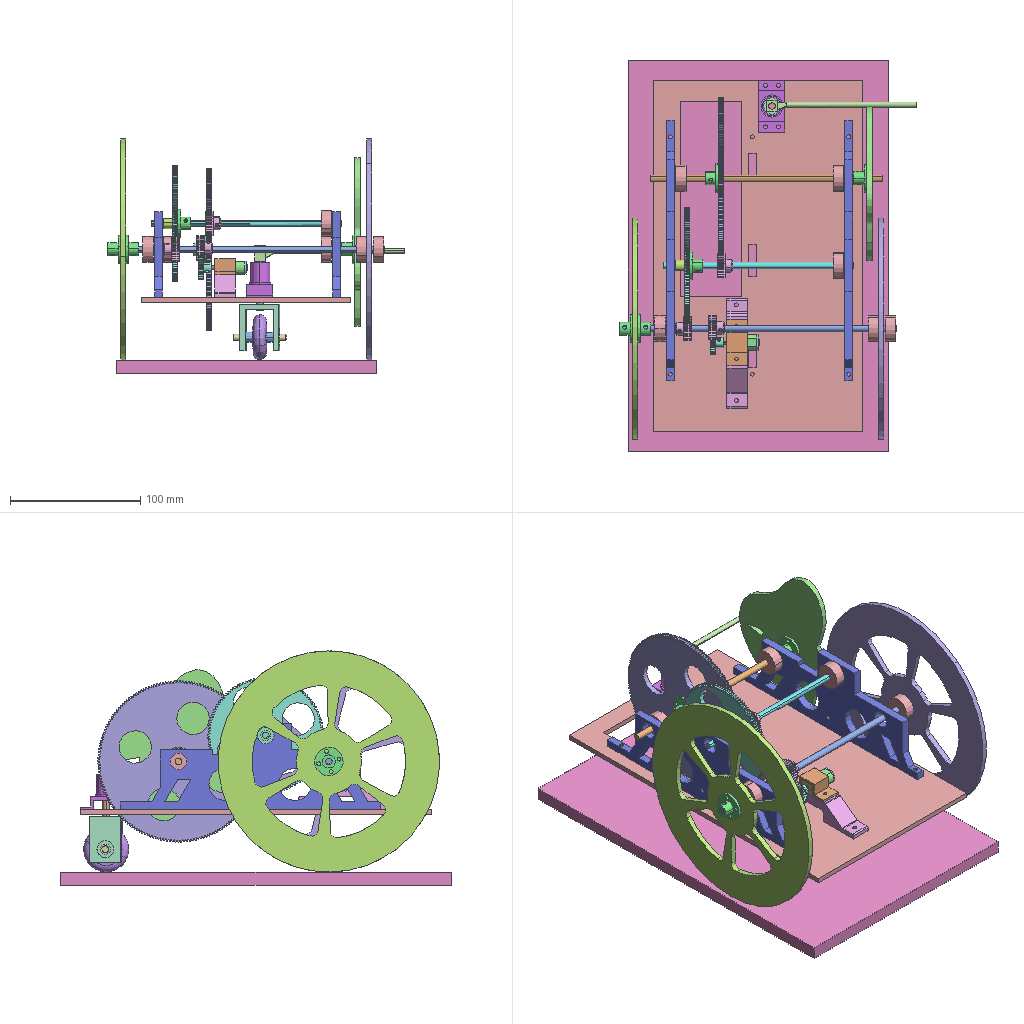Assembly | SolidWorks | 28 different items | 41 placed | box 228 x 300 x 180 mm
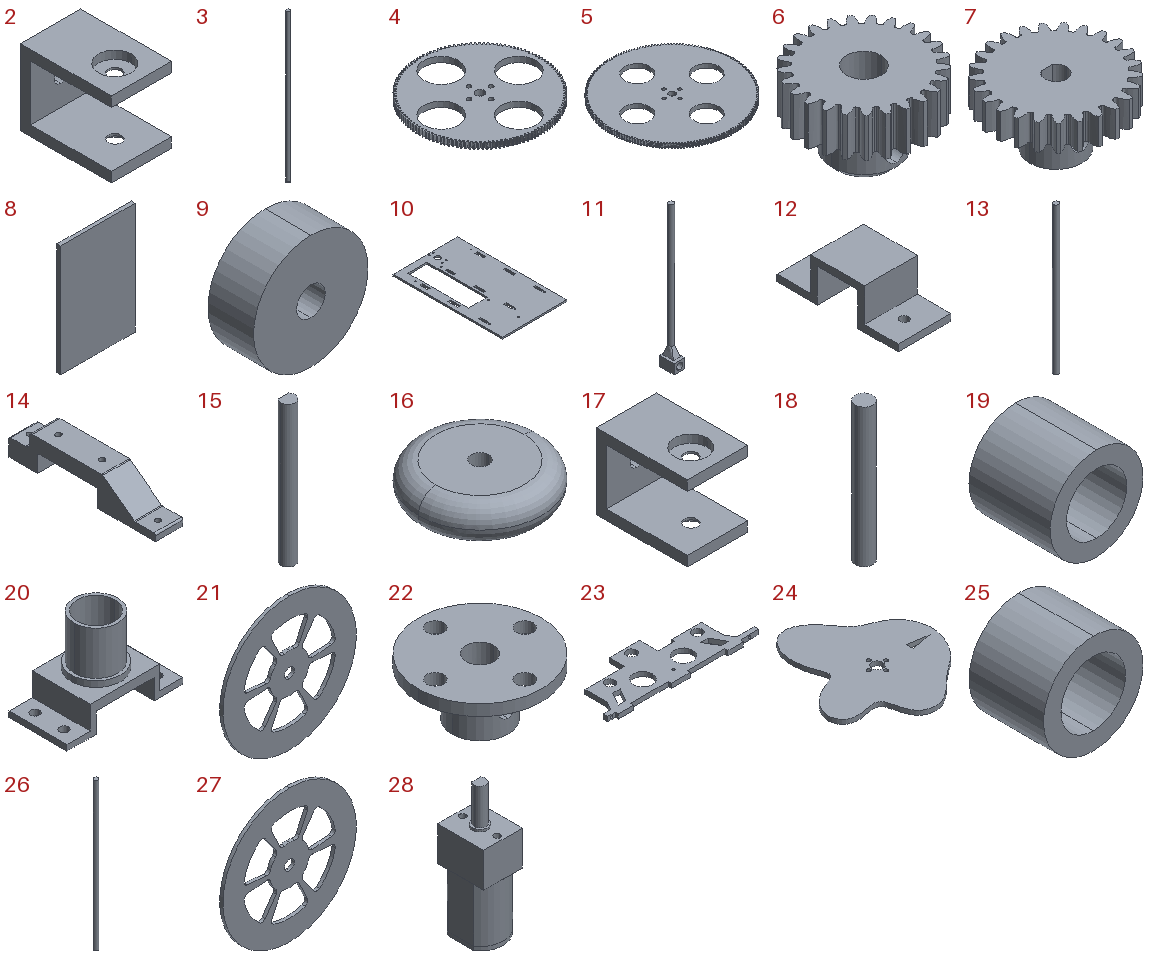Parts list (item | name | quantity | parent item | size | volume | features):
1 | (subassembly) | x1 | - | - | - | -
2 | (subassembly) | x1 | - | 23.897 x 36 x 30 mm | 8017 mm3 | -
3 | - | x1 | - | 5 x 5 x 213 mm | 3913 mm3 | features ICE 3, Extrusion 1
4 | - | x1 | - | 88.898 x 88.892 x 4 mm | 15932 mm3 | features ICE 8, CirPattern 1, Extrusion 1, RefAxis 1
5 | - | x1 | - | 123.899 x 123.895 x 4 mm | 39033 mm3 | features ICE 2, CirPattern 1, Extrusion 1, RefAxis 1
6 | - | x3 | - | 18.888 x 18.854 x 12 mm | 1581 mm3 | features ICE 6, Chamfer 1, CirPattern 1, Extrusion 1, RefAxis 1
7 | - | x1 | - | 18.888 x 18.854 x 10 mm | 1132 mm3 | features ICE 7, CirPattern 1, Extrusion 1, RefAxis 1
8 | - | x1 | - | 200 x 10 x 300 mm | 600000 mm3 | features Extrusion 1
9 | - | x6 | - | 20 x 8 x 20 mm | 2356 mm3 | features Extrusion 1
10 | - | x1 | - | 161 x 270 x 4 mm | 140085 mm3 | features ICE 34, FlatPattern 1, SMBaseFlange 1, SheetMetal 1
11 | - | x1 | - | 8.5 x 12 x 115 mm | 2022 mm3 | features ICE 4, Blend 1, Extrusion 1
12 | - | x1 | - | 15.7 x 36 x 12 mm | 1739 mm3 | features ICE 3, Extrusion 1, HoleWzd 1
13 | - | x1 | - | 5 x 5 x 146 mm | 2741 mm3 | features ICE 2, Extrusion 1
14 | - | x1 | - | 15.7 x 84.104 x 18.06 mm | 12021 mm3 | features ICE 11, Fillet 3, Extrusion 1
15 | - | x1 | - | 5 x 5 x 50 mm | 947.142 mm3 | features ICE 2, Extrusion 1
16 | - | x1 | - | 35 x 35 x 10 mm | 8320 mm3 | features Extrusion 1, Fillet 1, ICE 1
17 | - | x1 | in 2 | 23.897 x 36 x 30 mm | 8017 mm3 | features ICE 12, Extrusion 1, MirrorPattern 1
18 | - | x1 | - | 5 x 5 x 40 mm | 785.398 mm3 | features Extrusion 1
19 | - | x1 | - | 8 x 7 x 8 mm | 203.198 mm3 | features Extrusion 1
20 | - | x1 | - | 40 x 20 x 27 mm | 3033 mm3 | features ICE 9, Extrusion 1
21 | - | x1 | - | 170 x 4 x 170 mm | 60845 mm3 | features Extrusion 1, Fillet 1, ICE 1
22 | - | x5 | - | 22 x 22 x 10 mm | 1099 mm3 | features ICE 4, Extrusion 1
23 | - | x2 | - | 200 x 70 x 6 mm | 39858 mm3 | features ICE 11, Extrusion 1
24 | - | x1 | - | 117.822 x 129.451 x 4 mm | 34423 mm3 | features CurveInFile 1, Extrusion 1
25 | - | x2 | - | 8 x 6 x 8 mm | 174.17 mm3 | features Extrusion 1
26 | - | x1 | - | 5 x 5 x 178.5 mm | 3505 mm3 | features Extrusion 1
27 | - | x1 | - | 170 x 4 x 170 mm | 60862 mm3 | features Extrusion 1, Fillet 1, ICE 1
28 | - | x1 | - | 10 x 12 x 35 mm | 2719 mm3 | features MBimport 1
Mates (type | each side: item.copy, entity, surface, feature):
Coincident | 10.1 face plane Base-Flange1 | assembly face | 8 times
Coincident | 10.1 face plane Cut-Extrude1 | assembly face | 2 times
Coincident | 10.1 face | assembly face | 6 times
Coincident | assembly face | assembly face | 60 times
Concentric | assembly face | assembly face | 19 times
Concentric | assembly face | 3.1 face cylinder Boss-Extrude1 | 4 times
DistanceDim | 3.1 face plane Boss-Extrude1 | assembly face | 2 times
Concentric | 3.1 face cylinder Boss-Extrude1 | 27.1 face cylinder Boss-Extrude1
Concentric | 27.1 face cylinder Boss-Extrude1 | assembly face | 2 times
Coincident | 27.1 face plane Boss-Extrude1 | assembly face | 2 times
Concentric | 3.1 face cylinder Boss-Extrude1 | assembly face | 4 times
Concentric | 3.1 face cylinder Boss-Extrude1 | 6.1 face cylinder Cut-Extrude6
Coincident | assembly face | 6.1 face plane Boss-Extrude3
Coincident | 4.1 face plane Cut-Extrude2 | assembly face
Concentric | assembly face | 26.1 face cylinder Boss-Extrude1 | 4 times
DistanceDim | 26.1 face plane Boss-Extrude1 | assembly face
Coincident | assembly face | 6.2 face plane Boss-Extrude3
Coincident | 3.1 face plane Boss-Extrude1 | assembly face
Coincident | 10.1 face plane Cut-Extrude8 | assembly face | 2 times
Coincident | 6.2 face plane Boss-Extrude3 | assembly face
Concentric | 10.1 face | assembly face | 4 times
Concentric | 20.1 face cylinder Boss-Extrude1 | assembly face
Coincident | 20.1 face plane Boss-Extrude1 | assembly face
Concentric | assembly face | 15.1 face cylinder Boss-Extrude1
Coincident | 10.1 face plane Base-Flange1 | 23.1 face plane Cut-Extrude1
Coincident | assembly face | 23.1 face plane Boss-Extrude1 | 6 times
Coincident | 10.1 face plane Base-Flange1 | 23.2 face plane Cut-Extrude1
Coincident | assembly face | 23.2 face plane Boss-Extrude1 | 6 times
Coincident | 6.1 face plane Boss-Extrude3 | assembly face
Concentric | assembly face | 23.2 face cylinder Boss-Extrude2
Perpendicular | 3.1 face plane Cut-Extrude2 | 6.1 axis
Perpendicular | 3.1 face plane Cut-Extrude2 | 6.3 axis
GearDim | 4.1 face cylinder Boss-Extrude1 | 6.1 face cylinder CirPattern1
DistanceDim | 26.1 face plane Boss-Extrude1 | 23.2 face plane Boss-Extrude1
Concentric | assembly face | 13.1 face cylinder Boss-Extrude1
Coincident | assembly face | 13.1 face plane Cut-Extrude2
Concentric | 6.2 face cylinder Boss-Extrude3 | 13.1 face cylinder Boss-Extrude1
Concentric | assembly face | 23.1 face cylinder Boss-Extrude2
Width | 10.1 face plane Cut-Extrude19 | 10.1 face plane Cut-Extrude20 | 8.1 face plane Boss-Extrude1 | 8.1 face plane Boss-Extrude1
Width | 18.1 face plane Boss-Extrude1 | 18.1 face plane Boss-Extrude1 | 17.1 face plane Boss-Extrude1 | 17.1 face plane Boss-Extrude1
Coincident | 17.1 face plane Boss-Extrude1 | assembly face | 2 times
Concentric | 18.1 face cylinder Boss-Extrude1 | assembly face | 2 times
Width | 10.1 face plane Cut-Extrude22 | 10.1 face plane Boss-Extrude12 | 8.1 face plane Boss-Extrude1 | 8.1 face plane Boss-Extrude1
Coincident | 10.1 face plane Cut-Extrude1 | 23.2 face plane Boss-Extrude1
Coincident | 18.1 face cylinder Boss-Extrude1 | 16.1 edge
Width | 17.1 face plane Boss-Extrude1 | 17.1 face plane Boss-Extrude1 | 16.1 face plane Boss-Extrude1 | 16.1 face plane Boss-Extrude1
Concentric | 3.1 face cylinder Boss-Extrude1 | 22.1 face cylinder Boss-Extrude2
DistanceDim | 27.1 face plane Boss-Extrude1 | 23.2 face plane Boss-Extrude1
Width | 3.1 face plane Boss-Extrude1 | 3.1 face plane Boss-Extrude1 | 21.1 face plane Boss-Extrude1 | 27.1 face plane Boss-Extrude1
Concentric | 3.1 face cylinder Boss-Extrude1 | 21.1 face cylinder Boss-Extrude1
Coincident | 27.1 face plane Boss-Extrude1 | 22.1 face plane Boss-Extrude1
Concentric | 3.1 face cylinder Boss-Extrude1 | 22.2 face cylinder Boss-Extrude2
Coincident | 27.1 face plane Boss-Extrude1 | 22.2 face plane Boss-Extrude1
Concentric | 22.3 face cylinder Cut-Extrude2 | 4.1 face cylinder Cut-Extrude7
Concentric | 4.1 face cylinder Boss-Extrude4 | 13.1 face cylinder Boss-Extrude1
Concentric | 13.1 face cylinder Boss-Extrude1 | 22.3 face cylinder Cut-Extrude1
DistanceDim | 4.1 face plane Boss-Extrude4 | 23.2 face plane Boss-Extrude1
Concentric | 26.1 face cylinder Boss-Extrude1 | 22.4 face cylinder Boss-Extrude2
Concentric | 26.1 face cylinder Boss-Extrude1 | 22.5 face cylinder Boss-Extrude2
Coincident | 4.1 face plane Cut-Extrude2 | 22.3 face plane Boss-Extrude1
Concentric | 3.1 face cylinder Boss-Extrude1 | 9.1 face cylinder Boss-Extrude1
DistanceDim | 21.1 face plane Boss-Extrude1 | 10.1 face plane Cut-Extrude20
Coincident | assembly face | 9.1 face plane Boss-Extrude1
Concentric | 13.1 face cylinder Boss-Extrude1 | 9.2 face cylinder Boss-Extrude1
Coincident | assembly face | 9.2 face plane Boss-Extrude1
Concentric | 26.1 face cylinder Boss-Extrude1 | 9.3 face cylinder Boss-Extrude1
Concentric | 26.1 face cylinder Boss-Extrude1 | 9.4 face cylinder Boss-Extrude1
Coincident | assembly face | 9.4 face plane Boss-Extrude1
Coincident | assembly face | 9.3 face plane Boss-Extrude1
Concentric | 18.1 face cylinder Boss-Extrude1 | 25.1 face cylinder Boss-Extrude1
Coincident | 17.1 face plane Cut-Extrude4 | 25.1 face plane Boss-Extrude1
Concentric | 18.1 face cylinder Boss-Extrude1 | 25.2 face cylinder Boss-Extrude1
Coincident | 17.1 face plane Cut-Extrude4 | 25.2 face plane Boss-Extrude1
Coincident | 4.1 face plane Boss-Extrude4 | 19.1 face plane Boss-Extrude1
Concentric | 13.1 face cylinder Boss-Extrude1 | 19.1 face cylinder Boss-Extrude1
Concentric | 3.1 face cylinder Boss-Extrude1 | 9.5 face cylinder Boss-Extrude1
Coincident | 10.1 face plane Base-Flange1 | 14.1 face plane Boss-Extrude10
Concentric | 14.1 edge | 12.1 edge | 2 times
Coincident | 14.1 face plane Boss-Extrude1 | 12.1 face plane Boss-Extrude2
Coincident | 28.1 face plane N20.step<1> | 12.1 face plane Boss-Extrude1
Coincident | 28.1 face plane N20.step<1> | 12.1 face plane Cut-Extrude1
Coincident | 28.1 face plane N20.step<1> | 12.1 face plane Boss-Extrude2
GearDim | 7.1 select_type:24 | 6.3 select_type:24
Width | 6.3 face plane Boss-Extrude1 | 6.3 face plane Boss-Extrude2 | 7.1 face plane Boss-Extrude1 | 7.1 face plane Boss-Extrude1
Concentric | 28.1 face cylinder N20.step<1> | 7.1 face cylinder Cut-Extrude7
DistanceDim | 7.1 face plane Boss-Extrude2 | 28.1 face plane N20.step<1>
Concentric | 10.1 edge | 14.1 face cylinder Cut-Extrude5
Concentric | 15.1 face cylinder Boss-Extrude1 | 11.1 face cylinder Cut-Extrude1
Coincident | 15.1 face plane Boss-Extrude1 | 11.1 face plane Boss-Extrude2
Coincident | 10.1 face plane Base-Flange1 | 20.1 face plane Boss-Extrude6
Concentric | 10.1 face cylinder Cut-Extrude31 | assembly face
Concentric | 10.1 face cylinder Cut-Extrude27 | 23.1 face cylinder Cut-Extrude6
Width | 6.2 face plane Boss-Extrude2 | 6.2 face plane Boss-Extrude1 | 5.1 face plane Boss-Extrude1 | 5.1 face plane Boss-Extrude1
Concentric | 10.1 face cylinder Cut-Extrude27 | 23.2 face cylinder Cut-Extrude6
Concentric | 26.1 face cylinder Boss-Extrude1 | 23.2 face cylinder Cut-Extrude7
Concentric | 22.4 face cylinder Cut-Extrude2 | 5.1 face cylinder Cut-Extrude2
Coincident | 22.4 face plane Boss-Extrude1 | 5.1 face plane Boss-Extrude1
Concentric | assembly face | 23.2 face cylinder Cut-Extrude7
DistanceDim | 5.1 face plane Boss-Extrude1 | 10.1 face plane Cut-Extrude9
Concentric | 26.1 face cylinder Boss-Extrude1 | 5.1 face cylinder Cut-Extrude2
GearDim | 5.1 select_type:24 | 6.2 select_type:24
Tangent | 27.1 face cylinder Boss-Extrude1 | 8.1 face plane Boss-Extrude1
Concentric | 26.1 face cylinder Boss-Extrude1 | 24.1 face cylinder Boss-Extrude1
Concentric | 22.5 face cylinder Cut-Extrude2 | 24.1 face cylinder Boss-Extrude1
Coincident | 22.5 face plane Boss-Extrude1 | 24.1 face plane Boss-Extrude1
Coincident | assembly face | 22.5 face plane Boss-Extrude2
Parallel | 11.1 select_type:24 | 24.1 select_type:24
Concentric | 15.1 face cylinder Boss-Extrude1 | assembly face
Parallel | 10.1 face plane Cut-Extrude22 | 20.1 face plane Boss-Extrude7
Tangent | 8.1 face plane Boss-Extrude1 | 16.1 edge
Concentric | 17.1 face cylinder Cut-Extrude13 | 15.1 face cylinder Boss-Extrude1
Concentric | 17.1 face cylinder Cut-Extrude14 | 18.1 face cylinder Boss-Extrude1
Coincident | 21.1 face plane Boss-Extrude1 | assembly face
Coincident | 21.1 edge | 9.5 face plane Boss-Extrude1
Concentric | 3.1 face cylinder Boss-Extrude1 | 9.6 face cylinder Boss-Extrude1
Coincident | assembly face | 9.6 face plane Boss-Extrude1